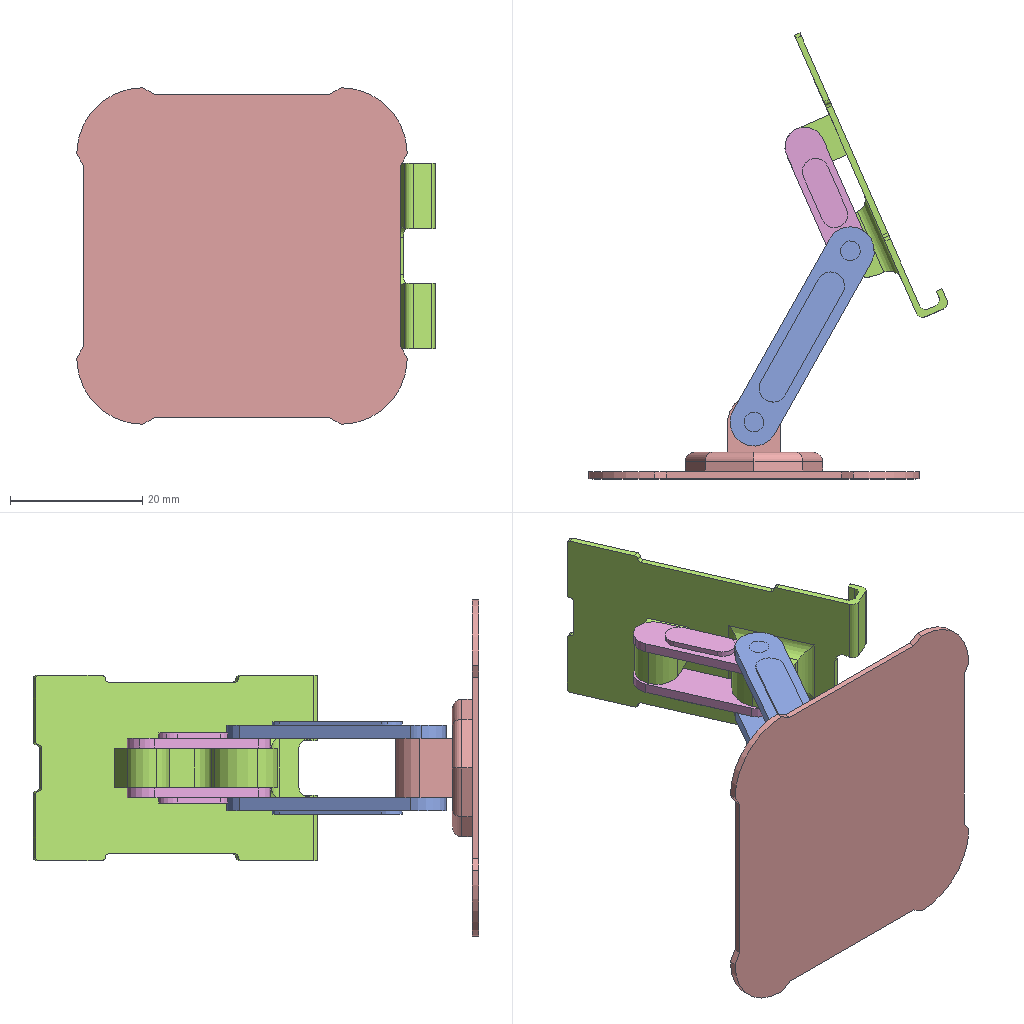Assembly | SolidWorks | 7 different items | 9 placed | box 54 x 67 x 51 mm
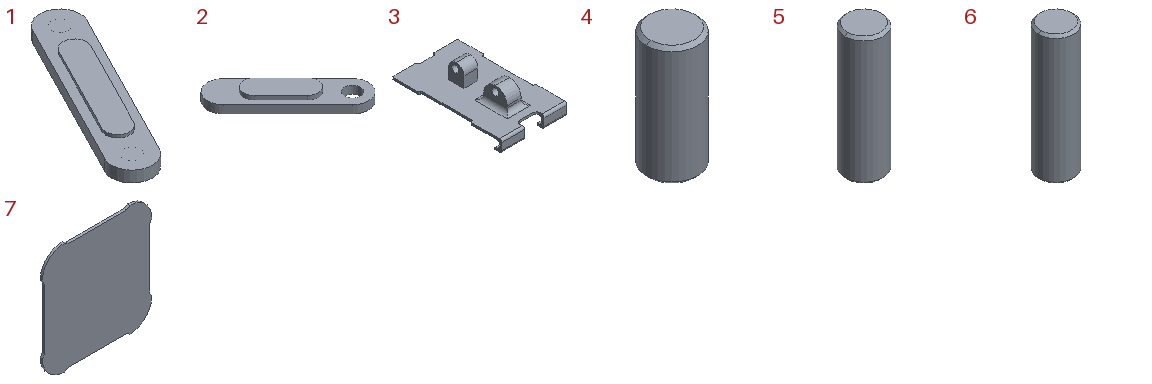Parts list (item | quantity | size | volume | features):
1 | x2 | 20.758 x 33.747 x 2.5 mm | 532.773 mm3 | features ICE 3, Extrusion 1
2 | x2 | 18.138 x 18.138 x 2.3 mm | 212.007 mm3 | features Cut 3, Extrusion 1, ICE 1
3 | x1 | 28 x 46.911 x 13 mm | 1866 mm3 | features Fillet 6, Cut 5, ICE 3, Extrusion 1, MirrorPattern 1
4 | x1 | 3 x 3 x 7 mm | 49.12 mm3 | features Chamfer 1, Extrusion 1
5 | x1 | 3 x 3 x 10 mm | 70.326 mm3 | features Chamfer 1, Extrusion 1
6 | x1 | 3 x 3 x 11 mm | 77.394 mm3 | features Chamfer 1, Extrusion 1
7 | x1 | 50 x 12.569 x 50.924 mm | 3739 mm3 | features ICE 2, Extrusion 1, Fillet 1
Mates (type | each side: item.copy, entity, surface, feature):
Concentric | 1.1 face cylinder Boss-Extrude1 | 3.1 face cylinder Cut-Extrude2
Concentric | 7.1 face cylinder Boss-Extrude3 | 1.2 face cylinder Boss-Extrude1
Concentric | 7.1 face cylinder Boss-Extrude3 | 1.1 face cylinder Boss-Extrude1
Coincident | 7.1 face plane Boss-Extrude3 | 1.1 face plane Boss-Extrude1
Coincident | 7.1 face plane Boss-Extrude3 | 1.2 face plane Boss-Extrude1
Concentric | 1.1 edge | 3.1 face cylinder Cut-Extrude2
Concentric | 1.2 face cylinder Boss-Extrude1 | 3.1 face cylinder Cut-Extrude2
Concentric | 1.1 edge | 2.1 edge
Coincident | 3.1 face plane Boss-Extrude2 | 2.1 face plane Boss-Extrude1
Coincident | 1.1 face plane Boss-Extrude1 | 2.1 face plane Boss-Extrude1
Concentric | 3.1 face cylinder Cut-Extrude10 | 2.1 edge
Concentric | 3.1 face cylinder Cut-Extrude2 | 2.2 edge
Concentric | 3.1 face cylinder Cut-Extrude10 | 2.2 edge
Coincident | 3.1 face plane Boss-Extrude4 | 2.2 face plane Boss-Extrude1
Concentric | 3.1 face cylinder Cut-Extrude10 | 4.1 face cylinder Boss-Extrude2
DistanceDim | 4.1 face plane Boss-Extrude2 | 2.2 face plane Boss-Extrude1
Concentric | 3.1 face cylinder Cut-Extrude2 | 5.1 face cylinder Boss-Extrude1
DistanceDim | 1.2 face plane Boss-Extrude1 | 5.1 face plane Boss-Extrude1
Concentric | 7.1 edge | 6.1 face cylinder Boss-Extrude1
DistanceDim | 6.1 face plane Boss-Extrude1 | 1.2 face plane Boss-Extrude1